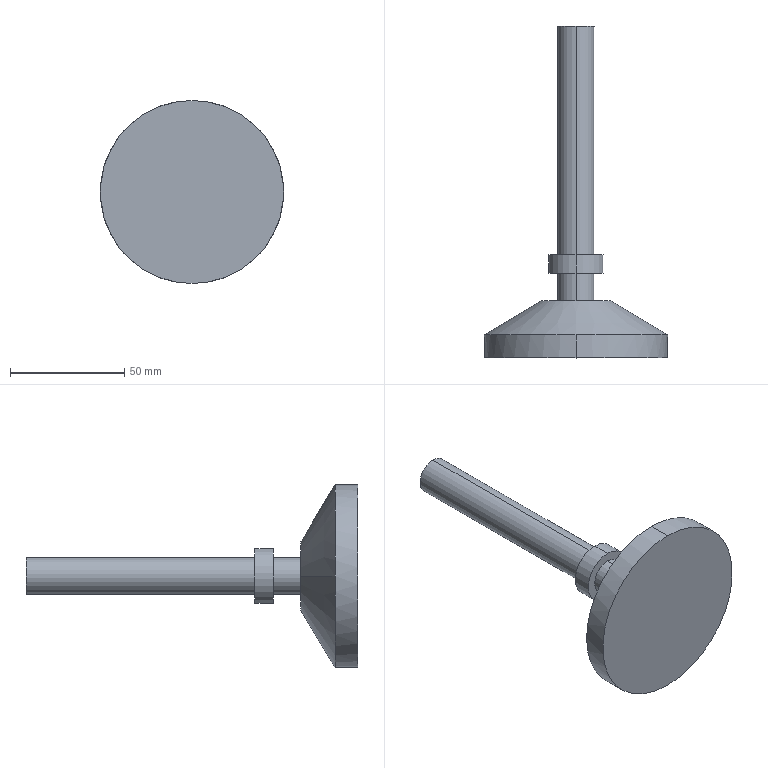Part | STEP file | Foot pad | 1 solid | 15 faces | box 80 x 145 x 80 mm | volume 114495 mm3 | cylinder 8 | plane 5 | cone 2 | commonest cylinder face diameters 16 x4 24 x2 80 x2
STEP:
#1=CARTESIAN_POINT('',(0.,0.,0.));
#2=DIRECTION('',(0.,0.,1.));
#3=DIRECTION('',(1.,0.,0.));
#4=AXIS2_PLACEMENT_3D('',#1,#2,#3);
#5=CARTESIAN_POINT('',(40.,10.,0.));
#6=VERTEX_POINT('',#5);
#7=CARTESIAN_POINT('',(0.,10.,40.));
#8=VERTEX_POINT('',#7);
#9=CARTESIAN_POINT('',(0.,10.,0.));
#10=DIRECTION('',(0.,-1.,0.));
#11=DIRECTION('',(0.,0.,-1.));
#12=AXIS2_PLACEMENT_3D('',#9,#10,#11);
#13=CIRCLE('',#12,40.);
#14=CARTESIAN_POINT('',(0.,0.,0.));
#15=DIRECTION('',(0.,-1.,0.));
#16=DIRECTION('',(0.,0.,-1.));
#17=AXIS2_PLACEMENT_3D('',#14,#15,#16);
#18=CYLINDRICAL_SURFACE('',#17,40.);
#19=CARTESIAN_POINT('',(0.,-10.));
#20=DIRECTION('',(1.,0.));
#21=VECTOR('',#20,1.);
#22=LINE('',#19,#21);
#23=(GEOMETRIC_REPRESENTATION_CONTEXT(2)PARAMETRIC_REPRESENTATION_CONTEXT()REPRESENTATION_CONTEXT('',''));
#24=DEFINITIONAL_REPRESENTATION('',(#22),#23);
#25=PCURVE('',#18,#24);
#26=CARTESIAN_POINT('',(0.,10.,0.));
#27=DIRECTION('',(0.,-1.,0.));
#28=DIRECTION('',(1.,0.,0.));
#29=AXIS2_PLACEMENT_3D('',#26,#27,#28);
#30=CONICAL_SURFACE('',#29,40.,1.03);
#31=CARTESIAN_POINT('',(-1.571,0.));
#32=DIRECTION('',(1.,0.));
#33=VECTOR('',#32,1.);
#34=LINE('',#31,#33);
#35=(GEOMETRIC_REPRESENTATION_CONTEXT(2)PARAMETRIC_REPRESENTATION_CONTEXT()REPRESENTATION_CONTEXT('',''));
#36=DEFINITIONAL_REPRESENTATION('',(#34),#35);
#37=PCURVE('',#30,#36);
#38=SURFACE_CURVE('',#13,(#25,#37),.PCURVE_S1.);
#39=EDGE_CURVE('',#6,#8,#38,.T.);
#40=ORIENTED_EDGE('',*,*,#39,.T.);
#41=CARTESIAN_POINT('',(0.,0.,40.));
#42=VERTEX_POINT('',#41);
#43=CARTESIAN_POINT('',(0.,0.,40.));
#44=DIRECTION('',(0.,-1.,0.));
#45=VECTOR('',#44,1.);
#46=LINE('',#43,#45);
#47=CARTESIAN_POINT('',(3.142,0.));
#48=DIRECTION('',(0.,1.));
#49=VECTOR('',#48,1.);
#50=LINE('',#47,#49);
#51=(GEOMETRIC_REPRESENTATION_CONTEXT(2)PARAMETRIC_REPRESENTATION_CONTEXT()REPRESENTATION_CONTEXT('',''));
#52=DEFINITIONAL_REPRESENTATION('',(#50),#51);
#53=PCURVE('',#18,#52);
#54=CARTESIAN_POINT('',(0.,0.,0.));
#55=DIRECTION('',(0.,-1.,0.));
#56=DIRECTION('',(0.,0.,-1.));
#57=AXIS2_PLACEMENT_3D('',#54,#55,#56);
#58=CYLINDRICAL_SURFACE('',#57,40.);
#59=CARTESIAN_POINT('',(3.142,0.));
#60=DIRECTION('',(0.,1.));
#61=VECTOR('',#60,1.);
#62=LINE('',#59,#61);
#63=(GEOMETRIC_REPRESENTATION_CONTEXT(2)PARAMETRIC_REPRESENTATION_CONTEXT()REPRESENTATION_CONTEXT('',''));
#64=DEFINITIONAL_REPRESENTATION('',(#62),#63);
#65=PCURVE('',#58,#64);
#66=SURFACE_CURVE('',#46,(#53,#65),.PCURVE_S1.);
#67=EDGE_CURVE('',#8,#42,#66,.T.);
#68=ORIENTED_EDGE('',*,*,#67,.T.);
#69=CARTESIAN_POINT('',(0.,0.,-40.));
#70=VERTEX_POINT('',#69);
#71=CARTESIAN_POINT('',(0.,0.,0.));
#72=DIRECTION('',(0.,-1.,0.));
#73=DIRECTION('',(0.,0.,-1.));
#74=AXIS2_PLACEMENT_3D('',#71,#72,#73);
#75=CIRCLE('',#74,40.);
#76=CARTESIAN_POINT('',(0.,0.));
#77=DIRECTION('',(1.,0.));
#78=VECTOR('',#77,1.);
#79=LINE('',#76,#78);
#80=(GEOMETRIC_REPRESENTATION_CONTEXT(2)PARAMETRIC_REPRESENTATION_CONTEXT()REPRESENTATION_CONTEXT('',''));
#81=DEFINITIONAL_REPRESENTATION('',(#79),#80);
#82=PCURVE('',#18,#81);
#83=CARTESIAN_POINT('',(0.,0.,0.));
#84=DIRECTION('',(0.,-1.,0.));
#85=DIRECTION('',(0.,0.,-1.));
#86=AXIS2_PLACEMENT_3D('',#83,#84,#85);
#87=PLANE('',#86);
#88=CARTESIAN_POINT('',(0.,0.));
#89=DIRECTION('',(1.,0.));
#90=AXIS2_PLACEMENT_2D('',#88,#89);
#91=CIRCLE('',#90,40.);
#92=(GEOMETRIC_REPRESENTATION_CONTEXT(2)PARAMETRIC_REPRESENTATION_CONTEXT()REPRESENTATION_CONTEXT('',''));
#93=DEFINITIONAL_REPRESENTATION('',(#91),#92);
#94=PCURVE('',#87,#93);
#95=SURFACE_CURVE('',#75,(#82,#94),.PCURVE_S1.);
#96=EDGE_CURVE('',#70,#42,#95,.T.);
#97=ORIENTED_EDGE('',*,*,#96,.F.);
#98=CARTESIAN_POINT('',(0.,10.,-40.));
#99=VERTEX_POINT('',#98);
#100=CARTESIAN_POINT('',(0.,0.,-40.));
#101=DIRECTION('',(0.,-1.,0.));
#102=VECTOR('',#101,1.);
#103=LINE('',#100,#102);
#104=CARTESIAN_POINT('',(0.,0.));
#105=DIRECTION('',(0.,1.));
#106=VECTOR('',#105,1.);
#107=LINE('',#104,#106);
#108=(GEOMETRIC_REPRESENTATION_CONTEXT(2)PARAMETRIC_REPRESENTATION_CONTEXT()REPRESENTATION_CONTEXT('',''));
#109=DEFINITIONAL_REPRESENTATION('',(#107),#108);
#110=PCURVE('',#18,#109);
#111=CARTESIAN_POINT('',(6.283,0.));
#112=DIRECTION('',(0.,1.));
#113=VECTOR('',#112,1.);
#114=LINE('',#111,#113);
#115=(GEOMETRIC_REPRESENTATION_CONTEXT(2)PARAMETRIC_REPRESENTATION_CONTEXT()REPRESENTATION_CONTEXT('',''));
#116=DEFINITIONAL_REPRESENTATION('',(#114),#115);
#117=PCURVE('',#58,#116);
#118=SURFACE_CURVE('',#103,(#110,#117),.PCURVE_S1.);
#119=EDGE_CURVE('',#99,#70,#118,.T.);
#120=ORIENTED_EDGE('',*,*,#119,.F.);
#121=CARTESIAN_POINT('',(0.,10.,0.));
#122=DIRECTION('',(0.,-1.,0.));
#123=DIRECTION('',(0.,0.,-1.));
#124=AXIS2_PLACEMENT_3D('',#121,#122,#123);
#125=CIRCLE('',#124,40.);
#126=CARTESIAN_POINT('',(0.,-10.));
#127=DIRECTION('',(1.,0.));
#128=VECTOR('',#127,1.);
#129=LINE('',#126,#128);
#130=(GEOMETRIC_REPRESENTATION_CONTEXT(2)PARAMETRIC_REPRESENTATION_CONTEXT()REPRESENTATION_CONTEXT('',''));
#131=DEFINITIONAL_REPRESENTATION('',(#129),#130);
#132=PCURVE('',#18,#131);
#133=CARTESIAN_POINT('',(0.,10.,0.));
#134=DIRECTION('',(0.,-1.,0.));
#135=DIRECTION('',(1.,0.,0.));
#136=AXIS2_PLACEMENT_3D('',#133,#134,#135);
#137=CONICAL_SURFACE('',#136,40.,1.03);
#138=CARTESIAN_POINT('',(4.712,0.));
#139=DIRECTION('',(1.,0.));
#140=VECTOR('',#139,1.);
#141=LINE('',#138,#140);
#142=(GEOMETRIC_REPRESENTATION_CONTEXT(2)PARAMETRIC_REPRESENTATION_CONTEXT()REPRESENTATION_CONTEXT('',''));
#143=DEFINITIONAL_REPRESENTATION('',(#141),#142);
#144=PCURVE('',#137,#143);
#145=SURFACE_CURVE('',#125,(#132,#144),.PCURVE_S1.);
#146=EDGE_CURVE('',#99,#6,#145,.T.);
#147=ORIENTED_EDGE('',*,*,#146,.T.);
#148=EDGE_LOOP('',(#40,#68,#97,#120,#147));
#149=FACE_BOUND('',#148,.T.);
#150=ADVANCED_FACE('',(#149),#18,.T.);
#151=CARTESIAN_POINT('',(15.,25.,0.));
#152=VERTEX_POINT('',#151);
#153=CARTESIAN_POINT('',(-15.,25.,0.));
#154=VERTEX_POINT('',#153);
#155=CARTESIAN_POINT('',(0.,25.,0.));
#156=DIRECTION('',(0.,-1.,0.));
#157=DIRECTION('',(1.,0.,0.));
#158=AXIS2_PLACEMENT_3D('',#155,#156,#157);
#159=CIRCLE('',#158,15.);
#160=CARTESIAN_POINT('',(0.,-15.));
#161=DIRECTION('',(1.,0.));
#162=VECTOR('',#161,1.);
#163=LINE('',#160,#162);
#164=(GEOMETRIC_REPRESENTATION_CONTEXT(2)PARAMETRIC_REPRESENTATION_CONTEXT()REPRESENTATION_CONTEXT('',''));
#165=DEFINITIONAL_REPRESENTATION('',(#163),#164);
#166=PCURVE('',#30,#165);
#167=CARTESIAN_POINT('',(8.,25.,0.));
#168=DIRECTION('',(0.,1.,0.));
#169=DIRECTION('',(0.,0.,1.));
#170=AXIS2_PLACEMENT_3D('',#167,#168,#169);
#171=PLANE('',#170);
#172=CARTESIAN_POINT('',(0.,7.));
#173=CARTESIAN_POINT('',(25.981,7.));
#174=CARTESIAN_POINT('',(12.99,-15.5));
#175=CARTESIAN_POINT('',(0.,-38.));
#176=CARTESIAN_POINT('',(-12.99,-15.5));
#177=CARTESIAN_POINT('',(-25.981,7.));
#178=CARTESIAN_POINT('',(0.,7.));
#179=(BOUNDED_CURVE()B_SPLINE_CURVE(2,(#172,#173,#174,#175,#176,#177,#178),.UNSPECIFIED.,.T.,.F.)B_SPLINE_CURVE_WITH_KNOTS((1,2,2,2,2,1),(-2.094,0.,2.094,4.189,6.283,8.378),.UNSPECIFIED.)CURVE()GEOMETRIC_REPRESENTATION_ITEM()RATIONAL_B_SPLINE_CURVE((1.,0.5,1.,0.5,1.,0.5,1.))REPRESENTATION_ITEM(''));
#180=(GEOMETRIC_REPRESENTATION_CONTEXT(2)PARAMETRIC_REPRESENTATION_CONTEXT()REPRESENTATION_CONTEXT('',''));
#181=DEFINITIONAL_REPRESENTATION('',(#179),#180);
#182=PCURVE('',#171,#181);
#183=SURFACE_CURVE('',#159,(#166,#182),.PCURVE_S1.);
#184=EDGE_CURVE('',#152,#154,#183,.T.);
#185=ORIENTED_EDGE('',*,*,#184,.T.);
#186=CARTESIAN_POINT('',(-40.,10.,0.));
#187=VERTEX_POINT('',#186);
#188=CARTESIAN_POINT('',(-40.,10.,0.));
#189=DIRECTION('',(-0.8575,-0.5145,0.));
#190=VECTOR('',#189,1.);
#191=LINE('',#188,#190);
#192=CARTESIAN_POINT('',(3.142,0.));
#193=DIRECTION('',(0.,1.));
#194=VECTOR('',#193,1.);
#195=LINE('',#192,#194);
#196=(GEOMETRIC_REPRESENTATION_CONTEXT(2)PARAMETRIC_REPRESENTATION_CONTEXT()REPRESENTATION_CONTEXT('',''));
#197=DEFINITIONAL_REPRESENTATION('',(#195),#196);
#198=PCURVE('',#30,#197);
#199=CARTESIAN_POINT('',(3.142,0.));
#200=DIRECTION('',(0.,1.));
#201=VECTOR('',#200,1.);
#202=LINE('',#199,#201);
#203=(GEOMETRIC_REPRESENTATION_CONTEXT(2)PARAMETRIC_REPRESENTATION_CONTEXT()REPRESENTATION_CONTEXT('',''));
#204=DEFINITIONAL_REPRESENTATION('',(#202),#203);
#205=PCURVE('',#137,#204);
#206=SURFACE_CURVE('',#191,(#198,#205),.PCURVE_S1.);
#207=EDGE_CURVE('',#154,#187,#206,.T.);
#208=ORIENTED_EDGE('',*,*,#207,.T.);
#209=CARTESIAN_POINT('',(0.,10.,0.));
#210=DIRECTION('',(0.,-1.,0.));
#211=DIRECTION('',(0.,0.,-1.));
#212=AXIS2_PLACEMENT_3D('',#209,#210,#211);
#213=CIRCLE('',#212,40.);
#214=CARTESIAN_POINT('',(-1.571,0.));
#215=DIRECTION('',(1.,0.));
#216=VECTOR('',#215,1.);
#217=LINE('',#214,#216);
#218=(GEOMETRIC_REPRESENTATION_CONTEXT(2)PARAMETRIC_REPRESENTATION_CONTEXT()REPRESENTATION_CONTEXT('',''));
#219=DEFINITIONAL_REPRESENTATION('',(#217),#218);
#220=PCURVE('',#30,#219);
#221=CARTESIAN_POINT('',(0.,-10.));
#222=DIRECTION('',(1.,0.));
#223=VECTOR('',#222,1.);
#224=LINE('',#221,#223);
#225=(GEOMETRIC_REPRESENTATION_CONTEXT(2)PARAMETRIC_REPRESENTATION_CONTEXT()REPRESENTATION_CONTEXT('',''));
#226=DEFINITIONAL_REPRESENTATION('',(#224),#225);
#227=PCURVE('',#58,#226);
#228=SURFACE_CURVE('',#213,(#220,#227),.PCURVE_S1.);
#229=EDGE_CURVE('',#8,#187,#228,.T.);
#230=ORIENTED_EDGE('',*,*,#229,.F.);
#231=ORIENTED_EDGE('',*,*,#39,.F.);
#232=CARTESIAN_POINT('',(40.,10.,0.));
#233=DIRECTION('',(0.8575,-0.5145,0.));
#234=VECTOR('',#233,1.);
#235=LINE('',#232,#234);
#236=CARTESIAN_POINT('',(0.,0.));
#237=DIRECTION('',(0.,1.));
#238=VECTOR('',#237,1.);
#239=LINE('',#236,#238);
#240=(GEOMETRIC_REPRESENTATION_CONTEXT(2)PARAMETRIC_REPRESENTATION_CONTEXT()REPRESENTATION_CONTEXT('',''));
#241=DEFINITIONAL_REPRESENTATION('',(#239),#240);
#242=PCURVE('',#30,#241);
#243=CARTESIAN_POINT('',(6.283,0.));
#244=DIRECTION('',(0.,1.));
#245=VECTOR('',#244,1.);
#246=LINE('',#243,#245);
#247=(GEOMETRIC_REPRESENTATION_CONTEXT(2)PARAMETRIC_REPRESENTATION_CONTEXT()REPRESENTATION_CONTEXT('',''));
#248=DEFINITIONAL_REPRESENTATION('',(#246),#247);
#249=PCURVE('',#137,#248);
#250=SURFACE_CURVE('',#235,(#242,#249),.PCURVE_S1.);
#251=EDGE_CURVE('',#152,#6,#250,.T.);
#252=ORIENTED_EDGE('',*,*,#251,.F.);
#253=EDGE_LOOP('',(#185,#208,#230,#231,#252));
#254=FACE_BOUND('',#253,.T.);
#255=ADVANCED_FACE('',(#254),#30,.T.);
#256=CARTESIAN_POINT('',(0.,37.,-8.));
#257=VERTEX_POINT('',#256);
#258=CARTESIAN_POINT('',(0.,37.,8.));
#259=VERTEX_POINT('',#258);
#260=CARTESIAN_POINT('',(0.,37.,0.));
#261=DIRECTION('',(0.,-1.,0.));
#262=DIRECTION('',(0.,0.,-1.));
#263=AXIS2_PLACEMENT_3D('',#260,#261,#262);
#264=CIRCLE('',#263,8.);
#265=CARTESIAN_POINT('',(0.,0.,0.));
#266=DIRECTION('',(0.,-1.,0.));
#267=DIRECTION('',(0.,0.,-1.));
#268=AXIS2_PLACEMENT_3D('',#265,#266,#267);
#269=CYLINDRICAL_SURFACE('',#268,8.);
#270=CARTESIAN_POINT('',(0.,-37.));
#271=DIRECTION('',(1.,0.));
#272=VECTOR('',#271,1.);
#273=LINE('',#270,#272);
#274=(GEOMETRIC_REPRESENTATION_CONTEXT(2)PARAMETRIC_REPRESENTATION_CONTEXT()REPRESENTATION_CONTEXT('',''));
#275=DEFINITIONAL_REPRESENTATION('',(#273),#274);
#276=PCURVE('',#269,#275);
#277=CARTESIAN_POINT('',(12.,37.,0.));
#278=DIRECTION('',(0.,-1.,0.));
#279=DIRECTION('',(0.,0.,-1.));
#280=AXIS2_PLACEMENT_3D('',#277,#278,#279);
#281=PLANE('',#280);
#282=CARTESIAN_POINT('',(0.,-12.));
#283=DIRECTION('',(1.,0.));
#284=AXIS2_PLACEMENT_2D('',#282,#283);
#285=CIRCLE('',#284,8.);
#286=(GEOMETRIC_REPRESENTATION_CONTEXT(2)PARAMETRIC_REPRESENTATION_CONTEXT()REPRESENTATION_CONTEXT('',''));
#287=DEFINITIONAL_REPRESENTATION('',(#285),#286);
#288=PCURVE('',#281,#287);
#289=SURFACE_CURVE('',#264,(#276,#288),.PCURVE_S1.);
#290=EDGE_CURVE('',#257,#259,#289,.T.);
#291=ORIENTED_EDGE('',*,*,#290,.T.);
#292=CARTESIAN_POINT('',(0.,25.,8.));
#293=VERTEX_POINT('',#292);
#294=CARTESIAN_POINT('',(0.,0.,8.));
#295=DIRECTION('',(0.,-1.,0.));
#296=VECTOR('',#295,1.);
#297=LINE('',#294,#296);
#298=CARTESIAN_POINT('',(3.142,0.));
#299=DIRECTION('',(0.,1.));
#300=VECTOR('',#299,1.);
#301=LINE('',#298,#300);
#302=(GEOMETRIC_REPRESENTATION_CONTEXT(2)PARAMETRIC_REPRESENTATION_CONTEXT()REPRESENTATION_CONTEXT('',''));
#303=DEFINITIONAL_REPRESENTATION('',(#301),#302);
#304=PCURVE('',#269,#303);
#305=CARTESIAN_POINT('',(0.,0.,0.));
#306=DIRECTION('',(0.,-1.,0.));
#307=DIRECTION('',(0.,0.,-1.));
#308=AXIS2_PLACEMENT_3D('',#305,#306,#307);
#309=CYLINDRICAL_SURFACE('',#308,8.);
#310=CARTESIAN_POINT('',(3.142,0.));
#311=DIRECTION('',(0.,1.));
#312=VECTOR('',#311,1.);
#313=LINE('',#310,#312);
#314=(GEOMETRIC_REPRESENTATION_CONTEXT(2)PARAMETRIC_REPRESENTATION_CONTEXT()REPRESENTATION_CONTEXT('',''));
#315=DEFINITIONAL_REPRESENTATION('',(#313),#314);
#316=PCURVE('',#309,#315);
#317=SURFACE_CURVE('',#297,(#304,#316),.PCURVE_S1.);
#318=EDGE_CURVE('',#259,#293,#317,.T.);
#319=ORIENTED_EDGE('',*,*,#318,.T.);
#320=CARTESIAN_POINT('',(0.,25.,-8.));
#321=VERTEX_POINT('',#320);
#322=CARTESIAN_POINT('',(0.,25.,0.));
#323=DIRECTION('',(0.,-1.,0.));
#324=DIRECTION('',(0.,0.,-1.));
#325=AXIS2_PLACEMENT_3D('',#322,#323,#324);
#326=CIRCLE('',#325,8.);
#327=CARTESIAN_POINT('',(0.,-25.));
#328=DIRECTION('',(1.,0.));
#329=VECTOR('',#328,1.);
#330=LINE('',#327,#329);
#331=(GEOMETRIC_REPRESENTATION_CONTEXT(2)PARAMETRIC_REPRESENTATION_CONTEXT()REPRESENTATION_CONTEXT('',''));
#332=DEFINITIONAL_REPRESENTATION('',(#330),#331);
#333=PCURVE('',#269,#332);
#334=CARTESIAN_POINT('',(-8.,-8.));
#335=CARTESIAN_POINT('',(-8.,5.856));
#336=CARTESIAN_POINT('',(4.,-1.072));
#337=CARTESIAN_POINT('',(16.,-8.));
#338=CARTESIAN_POINT('',(4.,-14.928));
#339=CARTESIAN_POINT('',(-8.,-21.856));
#340=CARTESIAN_POINT('',(-8.,-8.));
#341=(BOUNDED_CURVE()B_SPLINE_CURVE(2,(#334,#335,#336,#337,#338,#339,#340),.UNSPECIFIED.,.T.,.F.)B_SPLINE_CURVE_WITH_KNOTS((1,2,2,2,2,1),(-2.094,0.,2.094,4.189,6.283,8.378),.UNSPECIFIED.)CURVE()GEOMETRIC_REPRESENTATION_ITEM()RATIONAL_B_SPLINE_CURVE((1.,0.5,1.,0.5,1.,0.5,1.))REPRESENTATION_ITEM(''));
#342=(GEOMETRIC_REPRESENTATION_CONTEXT(2)PARAMETRIC_REPRESENTATION_CONTEXT()REPRESENTATION_CONTEXT('',''));
#343=DEFINITIONAL_REPRESENTATION('',(#341),#342);
#344=PCURVE('',#171,#343);
#345=SURFACE_CURVE('',#326,(#333,#344),.PCURVE_S1.);
#346=EDGE_CURVE('',#321,#293,#345,.T.);
#347=ORIENTED_EDGE('',*,*,#346,.F.);
#348=CARTESIAN_POINT('',(0.,0.,-8.));
#349=DIRECTION('',(0.,-1.,0.));
#350=VECTOR('',#349,1.);
#351=LINE('',#348,#350);
#352=CARTESIAN_POINT('',(0.,0.));
#353=DIRECTION('',(0.,1.));
#354=VECTOR('',#353,1.);
#355=LINE('',#352,#354);
#356=(GEOMETRIC_REPRESENTATION_CONTEXT(2)PARAMETRIC_REPRESENTATION_CONTEXT()REPRESENTATION_CONTEXT('',''));
#357=DEFINITIONAL_REPRESENTATION('',(#355),#356);
#358=PCURVE('',#269,#357);
#359=CARTESIAN_POINT('',(6.283,0.));
#360=DIRECTION('',(0.,1.));
#361=VECTOR('',#360,1.);
#362=LINE('',#359,#361);
#363=(GEOMETRIC_REPRESENTATION_CONTEXT(2)PARAMETRIC_REPRESENTATION_CONTEXT()REPRESENTATION_CONTEXT('',''));
#364=DEFINITIONAL_REPRESENTATION('',(#362),#363);
#365=PCURVE('',#309,#364);
#366=SURFACE_CURVE('',#351,(#358,#365),.PCURVE_S1.);
#367=EDGE_CURVE('',#257,#321,#366,.T.);
#368=ORIENTED_EDGE('',*,*,#367,.F.);
#369=EDGE_LOOP('',(#291,#319,#347,#368));
#370=FACE_BOUND('',#369,.T.);
#371=ADVANCED_FACE('',(#370),#269,.T.);
#372=CARTESIAN_POINT('',(0.,45.,-12.));
#373=VERTEX_POINT('',#372);
#374=CARTESIAN_POINT('',(0.,45.,12.));
#375=VERTEX_POINT('',#374);
#376=CARTESIAN_POINT('',(0.,45.,0.));
#377=DIRECTION('',(0.,-1.,0.));
#378=DIRECTION('',(0.,0.,-1.));
#379=AXIS2_PLACEMENT_3D('',#376,#377,#378);
#380=CIRCLE('',#379,12.);
#381=CARTESIAN_POINT('',(0.,0.,0.));
#382=DIRECTION('',(0.,-1.,0.));
#383=DIRECTION('',(0.,0.,-1.));
#384=AXIS2_PLACEMENT_3D('',#381,#382,#383);
#385=CYLINDRICAL_SURFACE('',#384,12.);
#386=CARTESIAN_POINT('',(0.,-45.));
#387=DIRECTION('',(1.,0.));
#388=VECTOR('',#387,1.);
#389=LINE('',#386,#388);
#390=(GEOMETRIC_REPRESENTATION_CONTEXT(2)PARAMETRIC_REPRESENTATION_CONTEXT()REPRESENTATION_CONTEXT('',''));
#391=DEFINITIONAL_REPRESENTATION('',(#389),#390);
#392=PCURVE('',#385,#391);
#393=CARTESIAN_POINT('',(8.,45.,0.));
#394=DIRECTION('',(0.,1.,0.));
#395=DIRECTION('',(0.,0.,1.));
#396=AXIS2_PLACEMENT_3D('',#393,#394,#395);
#397=PLANE('',#396);
#398=CARTESIAN_POINT('',(-12.,-8.));
#399=CARTESIAN_POINT('',(-12.,12.785));
#400=CARTESIAN_POINT('',(6.,2.392));
#401=CARTESIAN_POINT('',(24.,-8.));
#402=CARTESIAN_POINT('',(6.,-18.392));
#403=CARTESIAN_POINT('',(-12.,-28.785));
#404=CARTESIAN_POINT('',(-12.,-8.));
#405=(BOUNDED_CURVE()B_SPLINE_CURVE(2,(#398,#399,#400,#401,#402,#403,#404),.UNSPECIFIED.,.T.,.F.)B_SPLINE_CURVE_WITH_KNOTS((1,2,2,2,2,1),(-2.094,0.,2.094,4.189,6.283,8.378),.UNSPECIFIED.)CURVE()GEOMETRIC_REPRESENTATION_ITEM()RATIONAL_B_SPLINE_CURVE((1.,0.5,1.,0.5,1.,0.5,1.))REPRESENTATION_ITEM(''));
#406=(GEOMETRIC_REPRESENTATION_CONTEXT(2)PARAMETRIC_REPRESENTATION_CONTEXT()REPRESENTATION_CONTEXT('',''));
#407=DEFINITIONAL_REPRESENTATION('',(#405),#406);
#408=PCURVE('',#397,#407);
#409=SURFACE_CURVE('',#380,(#392,#408),.PCURVE_S1.);
#410=EDGE_CURVE('',#373,#375,#409,.T.);
#411=ORIENTED_EDGE('',*,*,#410,.T.);
#412=CARTESIAN_POINT('',(0.,37.,12.));
#413=VERTEX_POINT('',#412);
#414=CARTESIAN_POINT('',(0.,0.,12.));
#415=DIRECTION('',(0.,-1.,0.));
#416=VECTOR('',#415,1.);
#417=LINE('',#414,#416);
#418=CARTESIAN_POINT('',(3.142,0.));
#419=DIRECTION('',(0.,1.));
#420=VECTOR('',#419,1.);
#421=LINE('',#418,#420);
#422=(GEOMETRIC_REPRESENTATION_CONTEXT(2)PARAMETRIC_REPRESENTATION_CONTEXT()REPRESENTATION_CONTEXT('',''));
#423=DEFINITIONAL_REPRESENTATION('',(#421),#422);
#424=PCURVE('',#385,#423);
#425=CARTESIAN_POINT('',(0.,0.,0.));
#426=DIRECTION('',(0.,-1.,0.));
#427=DIRECTION('',(0.,0.,-1.));
#428=AXIS2_PLACEMENT_3D('',#425,#426,#427);
#429=CYLINDRICAL_SURFACE('',#428,12.);
#430=CARTESIAN_POINT('',(3.142,0.));
#431=DIRECTION('',(0.,1.));
#432=VECTOR('',#431,1.);
#433=LINE('',#430,#432);
#434=(GEOMETRIC_REPRESENTATION_CONTEXT(2)PARAMETRIC_REPRESENTATION_CONTEXT()REPRESENTATION_CONTEXT('',''));
#435=DEFINITIONAL_REPRESENTATION('',(#433),#434);
#436=PCURVE('',#429,#435);
#437=SURFACE_CURVE('',#417,(#424,#436),.PCURVE_S1.);
#438=EDGE_CURVE('',#375,#413,#437,.T.);
#439=ORIENTED_EDGE('',*,*,#438,.T.);
#440=CARTESIAN_POINT('',(0.,37.,-12.));
#441=VERTEX_POINT('',#440);
#442=CARTESIAN_POINT('',(0.,37.,0.));
#443=DIRECTION('',(0.,-1.,0.));
#444=DIRECTION('',(0.,0.,-1.));
#445=AXIS2_PLACEMENT_3D('',#442,#443,#444);
#446=CIRCLE('',#445,12.);
#447=CARTESIAN_POINT('',(0.,-37.));
#448=DIRECTION('',(1.,0.));
#449=VECTOR('',#448,1.);
#450=LINE('',#447,#449);
#451=(GEOMETRIC_REPRESENTATION_CONTEXT(2)PARAMETRIC_REPRESENTATION_CONTEXT()REPRESENTATION_CONTEXT('',''));
#452=DEFINITIONAL_REPRESENTATION('',(#450),#451);
#453=PCURVE('',#385,#452);
#454=CARTESIAN_POINT('',(0.,-12.));
#455=DIRECTION('',(1.,0.));
#456=AXIS2_PLACEMENT_2D('',#454,#455);
#457=CIRCLE('',#456,12.);
#458=(GEOMETRIC_REPRESENTATION_CONTEXT(2)PARAMETRIC_REPRESENTATION_CONTEXT()REPRESENTATION_CONTEXT('',''));
#459=DEFINITIONAL_REPRESENTATION('',(#457),#458);
#460=PCURVE('',#281,#459);
#461=SURFACE_CURVE('',#446,(#453,#460),.PCURVE_S1.);
#462=EDGE_CURVE('',#441,#413,#461,.T.);
#463=ORIENTED_EDGE('',*,*,#462,.F.);
#464=CARTESIAN_POINT('',(0.,0.,-12.));
#465=DIRECTION('',(0.,-1.,0.));
#466=VECTOR('',#465,1.);
#467=LINE('',#464,#466);
#468=CARTESIAN_POINT('',(0.,0.));
#469=DIRECTION('',(0.,1.));
#470=VECTOR('',#469,1.);
#471=LINE('',#468,#470);
#472=(GEOMETRIC_REPRESENTATION_CONTEXT(2)PARAMETRIC_REPRESENTATION_CONTEXT()REPRESENTATION_CONTEXT('',''));
#473=DEFINITIONAL_REPRESENTATION('',(#471),#472);
#474=PCURVE('',#385,#473);
#475=CARTESIAN_POINT('',(6.283,0.));
#476=DIRECTION('',(0.,1.));
#477=VECTOR('',#476,1.);
#478=LINE('',#475,#477);
#479=(GEOMETRIC_REPRESENTATION_CONTEXT(2)PARAMETRIC_REPRESENTATION_CONTEXT()REPRESENTATION_CONTEXT('',''));
#480=DEFINITIONAL_REPRESENTATION('',(#478),#479);
#481=PCURVE('',#429,#480);
#482=SURFACE_CURVE('',#467,(#474,#481),.PCURVE_S1.);
#483=EDGE_CURVE('',#373,#441,#482,.T.);
#484=ORIENTED_EDGE('',*,*,#483,.F.);
#485=EDGE_LOOP('',(#411,#439,#463,#484));
#486=FACE_BOUND('',#485,.T.);
#487=ADVANCED_FACE('',(#486),#385,.T.);
#488=CARTESIAN_POINT('',(0.,145.,-8.));
#489=VERTEX_POINT('',#488);
#490=CARTESIAN_POINT('',(0.,145.,8.));
#491=VERTEX_POINT('',#490);
#492=CARTESIAN_POINT('',(0.,145.,0.));
#493=DIRECTION('',(0.,-1.,0.));
#494=DIRECTION('',(0.,0.,-1.));
#495=AXIS2_PLACEMENT_3D('',#492,#493,#494);
#496=CIRCLE('',#495,8.);
#497=CARTESIAN_POINT('',(0.,0.,0.));
#498=DIRECTION('',(0.,-1.,0.));
#499=DIRECTION('',(0.,0.,-1.));
#500=AXIS2_PLACEMENT_3D('',#497,#498,#499);
#501=CYLINDRICAL_SURFACE('',#500,8.);
#502=CARTESIAN_POINT('',(0.,-145.));
#503=DIRECTION('',(1.,0.));
#504=VECTOR('',#503,1.);
#505=LINE('',#502,#504);
#506=(GEOMETRIC_REPRESENTATION_CONTEXT(2)PARAMETRIC_REPRESENTATION_CONTEXT()REPRESENTATION_CONTEXT('',''));
#507=DEFINITIONAL_REPRESENTATION('',(#505),#506);
#508=PCURVE('',#501,#507);
#509=CARTESIAN_POINT('',(0.,145.,0.));
#510=DIRECTION('',(0.,1.,0.));
#511=DIRECTION('',(0.,0.,1.));
#512=AXIS2_PLACEMENT_3D('',#509,#510,#511);
#513=PLANE('',#512);
#514=CARTESIAN_POINT('',(-8.,0.));
#515=CARTESIAN_POINT('',(-8.,13.856));
#516=CARTESIAN_POINT('',(4.,6.928));
#517=CARTESIAN_POINT('',(16.,0.));
#518=CARTESIAN_POINT('',(4.,-6.928));
#519=CARTESIAN_POINT('',(-8.,-13.856));
#520=CARTESIAN_POINT('',(-8.,0.));
#521=(BOUNDED_CURVE()B_SPLINE_CURVE(2,(#514,#515,#516,#517,#518,#519,#520),.UNSPECIFIED.,.T.,.F.)B_SPLINE_CURVE_WITH_KNOTS((1,2,2,2,2,1),(-2.094,0.,2.094,4.189,6.283,8.378),.UNSPECIFIED.)CURVE()GEOMETRIC_REPRESENTATION_ITEM()RATIONAL_B_SPLINE_CURVE((1.,0.5,1.,0.5,1.,0.5,1.))REPRESENTATION_ITEM(''));
#522=(GEOMETRIC_REPRESENTATION_CONTEXT(2)PARAMETRIC_REPRESENTATION_CONTEXT()REPRESENTATION_CONTEXT('',''));
#523=DEFINITIONAL_REPRESENTATION('',(#521),#522);
#524=PCURVE('',#513,#523);
#525=SURFACE_CURVE('',#496,(#508,#524),.PCURVE_S1.);
#526=EDGE_CURVE('',#489,#491,#525,.T.);
#527=ORIENTED_EDGE('',*,*,#526,.T.);
#528=CARTESIAN_POINT('',(0.,45.,8.));
#529=VERTEX_POINT('',#528);
#530=CARTESIAN_POINT('',(0.,0.,8.));
#531=DIRECTION('',(0.,-1.,0.));
#532=VECTOR('',#531,1.);
#533=LINE('',#530,#532);
#534=CARTESIAN_POINT('',(3.142,0.));
#535=DIRECTION('',(0.,1.));
#536=VECTOR('',#535,1.);
#537=LINE('',#534,#536);
#538=(GEOMETRIC_REPRESENTATION_CONTEXT(2)PARAMETRIC_REPRESENTATION_CONTEXT()REPRESENTATION_CONTEXT('',''));
#539=DEFINITIONAL_REPRESENTATION('',(#537),#538);
#540=PCURVE('',#501,#539);
#541=CARTESIAN_POINT('',(0.,0.,0.));
#542=DIRECTION('',(0.,-1.,0.));
#543=DIRECTION('',(0.,0.,-1.));
#544=AXIS2_PLACEMENT_3D('',#541,#542,#543);
#545=CYLINDRICAL_SURFACE('',#544,8.);
#546=CARTESIAN_POINT('',(3.142,0.));
#547=DIRECTION('',(0.,1.));
#548=VECTOR('',#547,1.);
#549=LINE('',#546,#548);
#550=(GEOMETRIC_REPRESENTATION_CONTEXT(2)PARAMETRIC_REPRESENTATION_CONTEXT()REPRESENTATION_CONTEXT('',''));
#551=DEFINITIONAL_REPRESENTATION('',(#549),#550);
#552=PCURVE('',#545,#551);
#553=SURFACE_CURVE('',#533,(#540,#552),.PCURVE_S1.);
#554=EDGE_CURVE('',#491,#529,#553,.T.);
#555=ORIENTED_EDGE('',*,*,#554,.T.);
#556=CARTESIAN_POINT('',(0.,45.,-8.));
#557=VERTEX_POINT('',#556);
#558=CARTESIAN_POINT('',(0.,45.,0.));
#559=DIRECTION('',(0.,-1.,0.));
#560=DIRECTION('',(0.,0.,-1.));
#561=AXIS2_PLACEMENT_3D('',#558,#559,#560);
#562=CIRCLE('',#561,8.);
#563=CARTESIAN_POINT('',(0.,-45.));
#564=DIRECTION('',(1.,0.));
#565=VECTOR('',#564,1.);
#566=LINE('',#563,#565);
#567=(GEOMETRIC_REPRESENTATION_CONTEXT(2)PARAMETRIC_REPRESENTATION_CONTEXT()REPRESENTATION_CONTEXT('',''));
#568=DEFINITIONAL_REPRESENTATION('',(#566),#567);
#569=PCURVE('',#501,#568);
#570=CARTESIAN_POINT('',(-8.,-8.));
#571=CARTESIAN_POINT('',(-8.,5.856));
#572=CARTESIAN_POINT('',(4.,-1.072));
#573=CARTESIAN_POINT('',(16.,-8.));
#574=CARTESIAN_POINT('',(4.,-14.928));
#575=CARTESIAN_POINT('',(-8.,-21.856));
#576=CARTESIAN_POINT('',(-8.,-8.));
#577=(BOUNDED_CURVE()B_SPLINE_CURVE(2,(#570,#571,#572,#573,#574,#575,#576),.UNSPECIFIED.,.T.,.F.)B_SPLINE_CURVE_WITH_KNOTS((1,2,2,2,2,1),(-2.094,0.,2.094,4.189,6.283,8.378),.UNSPECIFIED.)CURVE()GEOMETRIC_REPRESENTATION_ITEM()RATIONAL_B_SPLINE_CURVE((1.,0.5,1.,0.5,1.,0.5,1.))REPRESENTATION_ITEM(''));
#578=(GEOMETRIC_REPRESENTATION_CONTEXT(2)PARAMETRIC_REPRESENTATION_CONTEXT()REPRESENTATION_CONTEXT('',''));
#579=DEFINITIONAL_REPRESENTATION('',(#577),#578);
#580=PCURVE('',#397,#579);
#581=SURFACE_CURVE('',#562,(#569,#580),.PCURVE_S1.);
#582=EDGE_CURVE('',#557,#529,#581,.T.);
#583=ORIENTED_EDGE('',*,*,#582,.F.);
#584=CARTESIAN_POINT('',(0.,0.,-8.));
#585=DIRECTION('',(0.,-1.,0.));
#586=VECTOR('',#585,1.);
#587=LINE('',#584,#586);
#588=CARTESIAN_POINT('',(0.,0.));
#589=DIRECTION('',(0.,1.));
#590=VECTOR('',#589,1.);
#591=LINE('',#588,#590);
#592=(GEOMETRIC_REPRESENTATION_CONTEXT(2)PARAMETRIC_REPRESENTATION_CONTEXT()REPRESENTATION_CONTEXT('',''));
#593=DEFINITIONAL_REPRESENTATION('',(#591),#592);
#594=PCURVE('',#501,#593);
#595=CARTESIAN_POINT('',(6.283,0.));
#596=DIRECTION('',(0.,1.));
#597=VECTOR('',#596,1.);
#598=LINE('',#595,#597);
#599=(GEOMETRIC_REPRESENTATION_CONTEXT(2)PARAMETRIC_REPRESENTATION_CONTEXT()REPRESENTATION_CONTEXT('',''));
#600=DEFINITIONAL_REPRESENTATION('',(#598),#599);
#601=PCURVE('',#545,#600);
#602=SURFACE_CURVE('',#587,(#594,#601),.PCURVE_S1.);
#603=EDGE_CURVE('',#489,#557,#602,.T.);
#604=ORIENTED_EDGE('',*,*,#603,.F.);
#605=EDGE_LOOP('',(#527,#555,#583,#604));
#606=FACE_BOUND('',#605,.T.);
#607=ADVANCED_FACE('',(#606),#501,.T.);
#608=ORIENTED_EDGE('',*,*,#96,.T.);
#609=CARTESIAN_POINT('',(0.,0.,0.));
#610=DIRECTION('',(0.,-1.,0.));
#611=DIRECTION('',(0.,0.,-1.));
#612=AXIS2_PLACEMENT_3D('',#609,#610,#611);
#613=CIRCLE('',#612,40.);
#614=CARTESIAN_POINT('',(0.,0.));
#615=DIRECTION('',(1.,0.));
#616=AXIS2_PLACEMENT_2D('',#614,#615);
#617=CIRCLE('',#616,40.);
#618=(GEOMETRIC_REPRESENTATION_CONTEXT(2)PARAMETRIC_REPRESENTATION_CONTEXT()REPRESENTATION_CONTEXT('',''));
#619=DEFINITIONAL_REPRESENTATION('',(#617),#618);
#620=PCURVE('',#87,#619);
#621=CARTESIAN_POINT('',(0.,0.));
#622=DIRECTION('',(1.,0.));
#623=VECTOR('',#622,1.);
#624=LINE('',#621,#623);
#625=(GEOMETRIC_REPRESENTATION_CONTEXT(2)PARAMETRIC_REPRESENTATION_CONTEXT()REPRESENTATION_CONTEXT('',''));
#626=DEFINITIONAL_REPRESENTATION('',(#624),#625);
#627=PCURVE('',#58,#626);
#628=SURFACE_CURVE('',#613,(#620,#627),.PCURVE_S1.);
#629=EDGE_CURVE('',#42,#70,#628,.T.);
#630=ORIENTED_EDGE('',*,*,#629,.T.);
#631=EDGE_LOOP('',(#608,#630));
#632=FACE_BOUND('',#631,.T.);
#633=ADVANCED_FACE('',(#632),#87,.T.);
#634=ORIENTED_EDGE('',*,*,#67,.F.);
#635=ORIENTED_EDGE('',*,*,#229,.T.);
#636=CARTESIAN_POINT('',(0.,10.,0.));
#637=DIRECTION('',(0.,-1.,0.));
#638=DIRECTION('',(0.,0.,-1.));
#639=AXIS2_PLACEMENT_3D('',#636,#637,#638);
#640=CIRCLE('',#639,40.);
#641=CARTESIAN_POINT('',(0.,-10.));
#642=DIRECTION('',(1.,0.));
#643=VECTOR('',#642,1.);
#644=LINE('',#641,#643);
#645=(GEOMETRIC_REPRESENTATION_CONTEXT(2)PARAMETRIC_REPRESENTATION_CONTEXT()REPRESENTATION_CONTEXT('',''));
#646=DEFINITIONAL_REPRESENTATION('',(#644),#645);
#647=PCURVE('',#58,#646);
#648=CARTESIAN_POINT('',(-1.571,0.));
#649=DIRECTION('',(1.,0.));
#650=VECTOR('',#649,1.);
#651=LINE('',#648,#650);
#652=(GEOMETRIC_REPRESENTATION_CONTEXT(2)PARAMETRIC_REPRESENTATION_CONTEXT()REPRESENTATION_CONTEXT('',''));
#653=DEFINITIONAL_REPRESENTATION('',(#651),#652);
#654=PCURVE('',#137,#653);
#655=SURFACE_CURVE('',#640,(#647,#654),.PCURVE_S1.);
#656=EDGE_CURVE('',#187,#99,#655,.T.);
#657=ORIENTED_EDGE('',*,*,#656,.T.);
#658=ORIENTED_EDGE('',*,*,#119,.T.);
#659=ORIENTED_EDGE('',*,*,#629,.F.);
#660=EDGE_LOOP('',(#634,#635,#657,#658,#659));
#661=FACE_BOUND('',#660,.T.);
#662=ADVANCED_FACE('',(#661),#58,.T.);
#663=ORIENTED_EDGE('',*,*,#207,.F.);
#664=CARTESIAN_POINT('',(0.,25.,0.));
#665=DIRECTION('',(0.,-1.,0.));
#666=DIRECTION('',(1.,0.,0.));
#667=AXIS2_PLACEMENT_3D('',#664,#665,#666);
#668=CIRCLE('',#667,15.);
#669=CARTESIAN_POINT('',(0.,-15.));
#670=DIRECTION('',(1.,0.));
#671=VECTOR('',#670,1.);
#672=LINE('',#669,#671);
#673=(GEOMETRIC_REPRESENTATION_CONTEXT(2)PARAMETRIC_REPRESENTATION_CONTEXT()REPRESENTATION_CONTEXT('',''));
#674=DEFINITIONAL_REPRESENTATION('',(#672),#673);
#675=PCURVE('',#137,#674);
#676=CARTESIAN_POINT('',(0.,7.));
#677=CARTESIAN_POINT('',(25.981,7.));
#678=CARTESIAN_POINT('',(12.99,-15.5));
#679=CARTESIAN_POINT('',(0.,-38.));
#680=CARTESIAN_POINT('',(-12.99,-15.5));
#681=CARTESIAN_POINT('',(-25.981,7.));
#682=CARTESIAN_POINT('',(0.,7.));
#683=(BOUNDED_CURVE()B_SPLINE_CURVE(2,(#676,#677,#678,#679,#680,#681,#682),.UNSPECIFIED.,.T.,.F.)B_SPLINE_CURVE_WITH_KNOTS((1,2,2,2,2,1),(-2.094,0.,2.094,4.189,6.283,8.378),.UNSPECIFIED.)CURVE()GEOMETRIC_REPRESENTATION_ITEM()RATIONAL_B_SPLINE_CURVE((1.,0.5,1.,0.5,1.,0.5,1.))REPRESENTATION_ITEM(''));
#684=(GEOMETRIC_REPRESENTATION_CONTEXT(2)PARAMETRIC_REPRESENTATION_CONTEXT()REPRESENTATION_CONTEXT('',''));
#685=DEFINITIONAL_REPRESENTATION('',(#683),#684);
#686=PCURVE('',#171,#685);
#687=SURFACE_CURVE('',#668,(#675,#686),.PCURVE_S1.);
#688=EDGE_CURVE('',#154,#152,#687,.T.);
#689=ORIENTED_EDGE('',*,*,#688,.T.);
#690=ORIENTED_EDGE('',*,*,#251,.T.);
#691=ORIENTED_EDGE('',*,*,#146,.F.);
#692=ORIENTED_EDGE('',*,*,#656,.F.);
#693=EDGE_LOOP('',(#663,#689,#690,#691,#692));
#694=FACE_BOUND('',#693,.T.);
#695=ADVANCED_FACE('',(#694),#137,.T.);
#696=ORIENTED_EDGE('',*,*,#184,.F.);
#697=ORIENTED_EDGE('',*,*,#688,.F.);
#698=EDGE_LOOP('',(#696,#697));
#699=FACE_BOUND('',#698,.T.);
#700=ORIENTED_EDGE('',*,*,#346,.T.);
#701=CARTESIAN_POINT('',(0.,25.,0.));
#702=DIRECTION('',(0.,-1.,0.));
#703=DIRECTION('',(0.,0.,-1.));
#704=AXIS2_PLACEMENT_3D('',#701,#702,#703);
#705=CIRCLE('',#704,8.);
#706=CARTESIAN_POINT('',(-8.,-8.));
#707=CARTESIAN_POINT('',(-8.,5.856));
#708=CARTESIAN_POINT('',(4.,-1.072));
#709=CARTESIAN_POINT('',(16.,-8.));
#710=CARTESIAN_POINT('',(4.,-14.928));
#711=CARTESIAN_POINT('',(-8.,-21.856));
#712=CARTESIAN_POINT('',(-8.,-8.));
#713=(BOUNDED_CURVE()B_SPLINE_CURVE(2,(#706,#707,#708,#709,#710,#711,#712),.UNSPECIFIED.,.T.,.F.)B_SPLINE_CURVE_WITH_KNOTS((1,2,2,2,2,1),(-2.094,0.,2.094,4.189,6.283,8.378),.UNSPECIFIED.)CURVE()GEOMETRIC_REPRESENTATION_ITEM()RATIONAL_B_SPLINE_CURVE((1.,0.5,1.,0.5,1.,0.5,1.))REPRESENTATION_ITEM(''));
#714=(GEOMETRIC_REPRESENTATION_CONTEXT(2)PARAMETRIC_REPRESENTATION_CONTEXT()REPRESENTATION_CONTEXT('',''));
#715=DEFINITIONAL_REPRESENTATION('',(#713),#714);
#716=PCURVE('',#171,#715);
#717=CARTESIAN_POINT('',(0.,-25.));
#718=DIRECTION('',(1.,0.));
#719=VECTOR('',#718,1.);
#720=LINE('',#717,#719);
#721=(GEOMETRIC_REPRESENTATION_CONTEXT(2)PARAMETRIC_REPRESENTATION_CONTEXT()REPRESENTATION_CONTEXT('',''));
#722=DEFINITIONAL_REPRESENTATION('',(#720),#721);
#723=PCURVE('',#309,#722);
#724=SURFACE_CURVE('',#705,(#716,#723),.PCURVE_S1.);
#725=EDGE_CURVE('',#293,#321,#724,.T.);
#726=ORIENTED_EDGE('',*,*,#725,.T.);
#727=EDGE_LOOP('',(#700,#726));
#728=FACE_BOUND('',#727,.T.);
#729=ADVANCED_FACE('',(#699,#728),#171,.T.);
#730=ORIENTED_EDGE('',*,*,#318,.F.);
#731=CARTESIAN_POINT('',(0.,37.,0.));
#732=DIRECTION('',(0.,-1.,0.));
#733=DIRECTION('',(0.,0.,-1.));
#734=AXIS2_PLACEMENT_3D('',#731,#732,#733);
#735=CIRCLE('',#734,8.);
#736=CARTESIAN_POINT('',(0.,-37.));
#737=DIRECTION('',(1.,0.));
#738=VECTOR('',#737,1.);
#739=LINE('',#736,#738);
#740=(GEOMETRIC_REPRESENTATION_CONTEXT(2)PARAMETRIC_REPRESENTATION_CONTEXT()REPRESENTATION_CONTEXT('',''));
#741=DEFINITIONAL_REPRESENTATION('',(#739),#740);
#742=PCURVE('',#309,#741);
#743=CARTESIAN_POINT('',(0.,-12.));
#744=DIRECTION('',(1.,0.));
#745=AXIS2_PLACEMENT_2D('',#743,#744);
#746=CIRCLE('',#745,8.);
#747=(GEOMETRIC_REPRESENTATION_CONTEXT(2)PARAMETRIC_REPRESENTATION_CONTEXT()REPRESENTATION_CONTEXT('',''));
#748=DEFINITIONAL_REPRESENTATION('',(#746),#747);
#749=PCURVE('',#281,#748);
#750=SURFACE_CURVE('',#735,(#742,#749),.PCURVE_S1.);
#751=EDGE_CURVE('',#259,#257,#750,.T.);
#752=ORIENTED_EDGE('',*,*,#751,.T.);
#753=ORIENTED_EDGE('',*,*,#367,.T.);
#754=ORIENTED_EDGE('',*,*,#725,.F.);
#755=EDGE_LOOP('',(#730,#752,#753,#754));
#756=FACE_BOUND('',#755,.T.);
#757=ADVANCED_FACE('',(#756),#309,.T.);
#758=ORIENTED_EDGE('',*,*,#290,.F.);
#759=ORIENTED_EDGE('',*,*,#751,.F.);
#760=EDGE_LOOP('',(#758,#759));
#761=FACE_BOUND('',#760,.T.);
#762=ORIENTED_EDGE('',*,*,#462,.T.);
#763=CARTESIAN_POINT('',(0.,37.,0.));
#764=DIRECTION('',(0.,-1.,0.));
#765=DIRECTION('',(0.,0.,-1.));
#766=AXIS2_PLACEMENT_3D('',#763,#764,#765);
#767=CIRCLE('',#766,12.);
#768=CARTESIAN_POINT('',(0.,-12.));
#769=DIRECTION('',(1.,0.));
#770=AXIS2_PLACEMENT_2D('',#768,#769);
#771=CIRCLE('',#770,12.);
#772=(GEOMETRIC_REPRESENTATION_CONTEXT(2)PARAMETRIC_REPRESENTATION_CONTEXT()REPRESENTATION_CONTEXT('',''));
#773=DEFINITIONAL_REPRESENTATION('',(#771),#772);
#774=PCURVE('',#281,#773);
#775=CARTESIAN_POINT('',(0.,-37.));
#776=DIRECTION('',(1.,0.));
#777=VECTOR('',#776,1.);
#778=LINE('',#775,#777);
#779=(GEOMETRIC_REPRESENTATION_CONTEXT(2)PARAMETRIC_REPRESENTATION_CONTEXT()REPRESENTATION_CONTEXT('',''));
#780=DEFINITIONAL_REPRESENTATION('',(#778),#779);
#781=PCURVE('',#429,#780);
#782=SURFACE_CURVE('',#767,(#774,#781),.PCURVE_S1.);
#783=EDGE_CURVE('',#413,#441,#782,.T.);
#784=ORIENTED_EDGE('',*,*,#783,.T.);
#785=EDGE_LOOP('',(#762,#784));
#786=FACE_BOUND('',#785,.T.);
#787=ADVANCED_FACE('',(#761,#786),#281,.T.);
#788=ORIENTED_EDGE('',*,*,#438,.F.);
#789=CARTESIAN_POINT('',(0.,45.,0.));
#790=DIRECTION('',(0.,-1.,0.));
#791=DIRECTION('',(0.,0.,-1.));
#792=AXIS2_PLACEMENT_3D('',#789,#790,#791);
#793=CIRCLE('',#792,12.);
#794=CARTESIAN_POINT('',(0.,-45.));
#795=DIRECTION('',(1.,0.));
#796=VECTOR('',#795,1.);
#797=LINE('',#794,#796);
#798=(GEOMETRIC_REPRESENTATION_CONTEXT(2)PARAMETRIC_REPRESENTATION_CONTEXT()REPRESENTATION_CONTEXT('',''));
#799=DEFINITIONAL_REPRESENTATION('',(#797),#798);
#800=PCURVE('',#429,#799);
#801=CARTESIAN_POINT('',(-12.,-8.));
#802=CARTESIAN_POINT('',(-12.,12.785));
#803=CARTESIAN_POINT('',(6.,2.392));
#804=CARTESIAN_POINT('',(24.,-8.));
#805=CARTESIAN_POINT('',(6.,-18.392));
#806=CARTESIAN_POINT('',(-12.,-28.785));
#807=CARTESIAN_POINT('',(-12.,-8.));
#808=(BOUNDED_CURVE()B_SPLINE_CURVE(2,(#801,#802,#803,#804,#805,#806,#807),.UNSPECIFIED.,.T.,.F.)B_SPLINE_CURVE_WITH_KNOTS((1,2,2,2,2,1),(-2.094,0.,2.094,4.189,6.283,8.378),.UNSPECIFIED.)CURVE()GEOMETRIC_REPRESENTATION_ITEM()RATIONAL_B_SPLINE_CURVE((1.,0.5,1.,0.5,1.,0.5,1.))REPRESENTATION_ITEM(''));
#809=(GEOMETRIC_REPRESENTATION_CONTEXT(2)PARAMETRIC_REPRESENTATION_CONTEXT()REPRESENTATION_CONTEXT('',''));
#810=DEFINITIONAL_REPRESENTATION('',(#808),#809);
#811=PCURVE('',#397,#810);
#812=SURFACE_CURVE('',#793,(#800,#811),.PCURVE_S1.);
#813=EDGE_CURVE('',#375,#373,#812,.T.);
#814=ORIENTED_EDGE('',*,*,#813,.T.);
#815=ORIENTED_EDGE('',*,*,#483,.T.);
#816=ORIENTED_EDGE('',*,*,#783,.F.);
#817=EDGE_LOOP('',(#788,#814,#815,#816));
#818=FACE_BOUND('',#817,.T.);
#819=ADVANCED_FACE('',(#818),#429,.T.);
#820=ORIENTED_EDGE('',*,*,#410,.F.);
#821=ORIENTED_EDGE('',*,*,#813,.F.);
#822=EDGE_LOOP('',(#820,#821));
#823=FACE_BOUND('',#822,.T.);
#824=ORIENTED_EDGE('',*,*,#582,.T.);
#825=CARTESIAN_POINT('',(0.,45.,0.));
#826=DIRECTION('',(0.,-1.,0.));
#827=DIRECTION('',(0.,0.,-1.));
#828=AXIS2_PLACEMENT_3D('',#825,#826,#827);
#829=CIRCLE('',#828,8.);
#830=CARTESIAN_POINT('',(-8.,-8.));
#831=CARTESIAN_POINT('',(-8.,5.856));
#832=CARTESIAN_POINT('',(4.,-1.072));
#833=CARTESIAN_POINT('',(16.,-8.));
#834=CARTESIAN_POINT('',(4.,-14.928));
#835=CARTESIAN_POINT('',(-8.,-21.856));
#836=CARTESIAN_POINT('',(-8.,-8.));
#837=(BOUNDED_CURVE()B_SPLINE_CURVE(2,(#830,#831,#832,#833,#834,#835,#836),.UNSPECIFIED.,.T.,.F.)B_SPLINE_CURVE_WITH_KNOTS((1,2,2,2,2,1),(-2.094,0.,2.094,4.189,6.283,8.378),.UNSPECIFIED.)CURVE()GEOMETRIC_REPRESENTATION_ITEM()RATIONAL_B_SPLINE_CURVE((1.,0.5,1.,0.5,1.,0.5,1.))REPRESENTATION_ITEM(''));
#838=(GEOMETRIC_REPRESENTATION_CONTEXT(2)PARAMETRIC_REPRESENTATION_CONTEXT()REPRESENTATION_CONTEXT('',''));
#839=DEFINITIONAL_REPRESENTATION('',(#837),#838);
#840=PCURVE('',#397,#839);
#841=CARTESIAN_POINT('',(0.,-45.));
#842=DIRECTION('',(1.,0.));
#843=VECTOR('',#842,1.);
#844=LINE('',#841,#843);
#845=(GEOMETRIC_REPRESENTATION_CONTEXT(2)PARAMETRIC_REPRESENTATION_CONTEXT()REPRESENTATION_CONTEXT('',''));
#846=DEFINITIONAL_REPRESENTATION('',(#844),#845);
#847=PCURVE('',#545,#846);
#848=SURFACE_CURVE('',#829,(#840,#847),.PCURVE_S1.);
#849=EDGE_CURVE('',#529,#557,#848,.T.);
#850=ORIENTED_EDGE('',*,*,#849,.T.);
#851=EDGE_LOOP('',(#824,#850));
#852=FACE_BOUND('',#851,.T.);
#853=ADVANCED_FACE('',(#823,#852),#397,.T.);
#854=ORIENTED_EDGE('',*,*,#554,.F.);
#855=CARTESIAN_POINT('',(0.,145.,0.));
#856=DIRECTION('',(0.,-1.,0.));
#857=DIRECTION('',(0.,0.,-1.));
#858=AXIS2_PLACEMENT_3D('',#855,#856,#857);
#859=CIRCLE('',#858,8.);
#860=CARTESIAN_POINT('',(0.,-145.));
#861=DIRECTION('',(1.,0.));
#862=VECTOR('',#861,1.);
#863=LINE('',#860,#862);
#864=(GEOMETRIC_REPRESENTATION_CONTEXT(2)PARAMETRIC_REPRESENTATION_CONTEXT()REPRESENTATION_CONTEXT('',''));
#865=DEFINITIONAL_REPRESENTATION('',(#863),#864);
#866=PCURVE('',#545,#865);
#867=CARTESIAN_POINT('',(-8.,0.));
#868=CARTESIAN_POINT('',(-8.,13.856));
#869=CARTESIAN_POINT('',(4.,6.928));
#870=CARTESIAN_POINT('',(16.,0.));
#871=CARTESIAN_POINT('',(4.,-6.928));
#872=CARTESIAN_POINT('',(-8.,-13.856));
#873=CARTESIAN_POINT('',(-8.,0.));
#874=(BOUNDED_CURVE()B_SPLINE_CURVE(2,(#867,#868,#869,#870,#871,#872,#873),.UNSPECIFIED.,.T.,.F.)B_SPLINE_CURVE_WITH_KNOTS((1,2,2,2,2,1),(-2.094,0.,2.094,4.189,6.283,8.378),.UNSPECIFIED.)CURVE()GEOMETRIC_REPRESENTATION_ITEM()RATIONAL_B_SPLINE_CURVE((1.,0.5,1.,0.5,1.,0.5,1.))REPRESENTATION_ITEM(''));
#875=(GEOMETRIC_REPRESENTATION_CONTEXT(2)PARAMETRIC_REPRESENTATION_CONTEXT()REPRESENTATION_CONTEXT('',''));
#876=DEFINITIONAL_REPRESENTATION('',(#874),#875);
#877=PCURVE('',#513,#876);
#878=SURFACE_CURVE('',#859,(#866,#877),.PCURVE_S1.);
#879=EDGE_CURVE('',#491,#489,#878,.T.);
#880=ORIENTED_EDGE('',*,*,#879,.T.);
#881=ORIENTED_EDGE('',*,*,#603,.T.);
#882=ORIENTED_EDGE('',*,*,#849,.F.);
#883=EDGE_LOOP('',(#854,#880,#881,#882));
#884=FACE_BOUND('',#883,.T.);
#885=ADVANCED_FACE('',(#884),#545,.T.);
#886=ORIENTED_EDGE('',*,*,#526,.F.);
#887=ORIENTED_EDGE('',*,*,#879,.F.);
#888=EDGE_LOOP('',(#886,#887));
#889=FACE_BOUND('',#888,.T.);
#890=ADVANCED_FACE('',(#889),#513,.T.);
#891=CLOSED_SHELL('',(#150,#255,#371,#487,#607,#633,#662,#695,#729,#757,#787,#819,#853,#885,#890));
#892=MANIFOLD_SOLID_BREP('',#891);
#893=(LENGTH_UNIT()NAMED_UNIT(*)SI_UNIT(.MILLI.,.METRE.));
#894=UNCERTAINTY_MEASURE_WITH_UNIT(LENGTH_MEASURE(0.0000001),#893,'','');
#895=(NAMED_UNIT(*)PLANE_ANGLE_UNIT()SI_UNIT($,.RADIAN.));
#896=(NAMED_UNIT(*)SI_UNIT($,.STERADIAN.)SOLID_ANGLE_UNIT());
#897=(GEOMETRIC_REPRESENTATION_CONTEXT(3)GLOBAL_UNCERTAINTY_ASSIGNED_CONTEXT((#894))GLOBAL_UNIT_ASSIGNED_CONTEXT((#893,#895,#896))REPRESENTATION_CONTEXT('',''));
#898=ADVANCED_BREP_SHAPE_REPRESENTATION('',(#4,#892),#897);